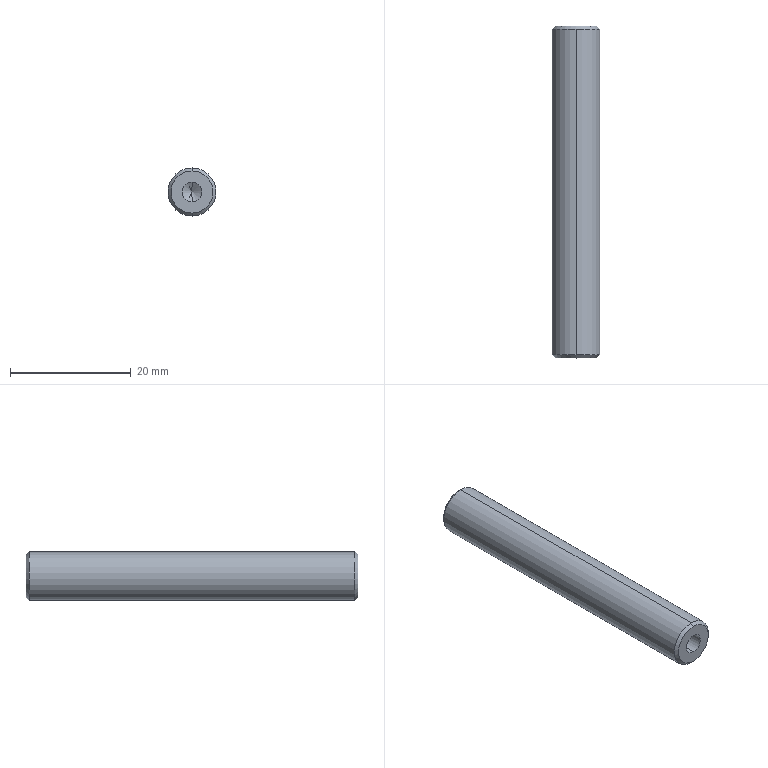Part | STEP file | PN_0012 | 1 solid | 16 faces | box 8 x 55 x 8 mm | volume 2556 mm3 | cone 8 | cylinder 6 | plane 2 | commonest cylinder face diameters 3.3 x4 8 x2
STEP:
#1=CARTESIAN_POINT('',(0.,0.,0.));
#2=DIRECTION('',(0.,0.,1.));
#3=DIRECTION('',(1.,0.,0.));
#4=AXIS2_PLACEMENT_3D('',#1,#2,#3);
#5=CARTESIAN_POINT('',(0.,27.5,3.5));
#6=VERTEX_POINT('',#5);
#7=CARTESIAN_POINT('',(0.,27.5,-3.5));
#8=VERTEX_POINT('',#7);
#9=CARTESIAN_POINT('',(0.,27.5,0.));
#10=DIRECTION('',(0.,1.,0.));
#11=DIRECTION('',(0.,0.,1.));
#12=AXIS2_PLACEMENT_3D('',#9,#10,#11);
#13=CIRCLE('',#12,3.5);
#14=CARTESIAN_POINT('',(0.,27.5,0.));
#15=DIRECTION('',(0.,-1.,0.));
#16=DIRECTION('',(0.,0.,-1.));
#17=AXIS2_PLACEMENT_3D('',#14,#15,#16);
#18=CONICAL_SURFACE('',#17,3.5,0.7854);
#19=CARTESIAN_POINT('',(3.142,0.));
#20=DIRECTION('',(-1.,0.));
#21=VECTOR('',#20,1.);
#22=LINE('',#19,#21);
#23=(GEOMETRIC_REPRESENTATION_CONTEXT(2)PARAMETRIC_REPRESENTATION_CONTEXT()REPRESENTATION_CONTEXT('',''));
#24=DEFINITIONAL_REPRESENTATION('',(#22),#23);
#25=PCURVE('',#18,#24);
#26=CARTESIAN_POINT('',(0.,27.5,0.));
#27=DIRECTION('',(0.,1.,0.));
#28=DIRECTION('',(0.,0.,1.));
#29=AXIS2_PLACEMENT_3D('',#26,#27,#28);
#30=PLANE('',#29);
#31=CARTESIAN_POINT('',(0.,0.));
#32=DIRECTION('',(1.,0.));
#33=AXIS2_PLACEMENT_2D('',#31,#32);
#34=CIRCLE('',#33,3.5);
#35=(GEOMETRIC_REPRESENTATION_CONTEXT(2)PARAMETRIC_REPRESENTATION_CONTEXT()REPRESENTATION_CONTEXT('',''));
#36=DEFINITIONAL_REPRESENTATION('',(#34),#35);
#37=PCURVE('',#30,#36);
#38=SURFACE_CURVE('',#13,(#25,#37),.PCURVE_S1.);
#39=EDGE_CURVE('',#6,#8,#38,.T.);
#40=ORIENTED_EDGE('',*,*,#39,.F.);
#41=CARTESIAN_POINT('',(0.,27.,4.));
#42=VERTEX_POINT('',#41);
#43=CARTESIAN_POINT('',(0.,27.5,3.5));
#44=DIRECTION('',(0.,-0.7071,0.7071));
#45=VECTOR('',#44,1.);
#46=LINE('',#43,#45);
#47=CARTESIAN_POINT('',(3.142,0.));
#48=DIRECTION('',(0.,1.));
#49=VECTOR('',#48,1.);
#50=LINE('',#47,#49);
#51=(GEOMETRIC_REPRESENTATION_CONTEXT(2)PARAMETRIC_REPRESENTATION_CONTEXT()REPRESENTATION_CONTEXT('',''));
#52=DEFINITIONAL_REPRESENTATION('',(#50),#51);
#53=PCURVE('',#18,#52);
#54=CARTESIAN_POINT('',(0.,27.5,0.));
#55=DIRECTION('',(0.,-1.,0.));
#56=DIRECTION('',(0.,0.,-1.));
#57=AXIS2_PLACEMENT_3D('',#54,#55,#56);
#58=CONICAL_SURFACE('',#57,3.5,0.7854);
#59=CARTESIAN_POINT('',(3.142,0.));
#60=DIRECTION('',(0.,1.));
#61=VECTOR('',#60,1.);
#62=LINE('',#59,#61);
#63=(GEOMETRIC_REPRESENTATION_CONTEXT(2)PARAMETRIC_REPRESENTATION_CONTEXT()REPRESENTATION_CONTEXT('',''));
#64=DEFINITIONAL_REPRESENTATION('',(#62),#63);
#65=PCURVE('',#58,#64);
#66=SURFACE_CURVE('',#46,(#53,#65),.PCURVE_S1.);
#67=EDGE_CURVE('',#6,#42,#66,.T.);
#68=ORIENTED_EDGE('',*,*,#67,.T.);
#69=CARTESIAN_POINT('',(0.,27.,-4.));
#70=VERTEX_POINT('',#69);
#71=CARTESIAN_POINT('',(0.,27.,0.));
#72=DIRECTION('',(0.,-1.,0.));
#73=DIRECTION('',(0.,0.,1.));
#74=AXIS2_PLACEMENT_3D('',#71,#72,#73);
#75=CIRCLE('',#74,4.);
#76=CARTESIAN_POINT('',(-3.142,0.5));
#77=DIRECTION('',(1.,0.));
#78=VECTOR('',#77,1.);
#79=LINE('',#76,#78);
#80=(GEOMETRIC_REPRESENTATION_CONTEXT(2)PARAMETRIC_REPRESENTATION_CONTEXT()REPRESENTATION_CONTEXT('',''));
#81=DEFINITIONAL_REPRESENTATION('',(#79),#80);
#82=PCURVE('',#18,#81);
#83=CARTESIAN_POINT('',(0.,27.5,0.));
#84=DIRECTION('',(0.,-1.,0.));
#85=DIRECTION('',(0.,0.,-1.));
#86=AXIS2_PLACEMENT_3D('',#83,#84,#85);
#87=CYLINDRICAL_SURFACE('',#86,4.);
#88=CARTESIAN_POINT('',(-3.142,0.5));
#89=DIRECTION('',(1.,0.));
#90=VECTOR('',#89,1.);
#91=LINE('',#88,#90);
#92=(GEOMETRIC_REPRESENTATION_CONTEXT(2)PARAMETRIC_REPRESENTATION_CONTEXT()REPRESENTATION_CONTEXT('',''));
#93=DEFINITIONAL_REPRESENTATION('',(#91),#92);
#94=PCURVE('',#87,#93);
#95=SURFACE_CURVE('',#75,(#82,#94),.PCURVE_S1.);
#96=EDGE_CURVE('',#70,#42,#95,.T.);
#97=ORIENTED_EDGE('',*,*,#96,.F.);
#98=CARTESIAN_POINT('',(0.,27.5,-3.5));
#99=DIRECTION('',(0.,-0.7071,-0.7071));
#100=VECTOR('',#99,1.);
#101=LINE('',#98,#100);
#102=CARTESIAN_POINT('',(0.,0.));
#103=DIRECTION('',(0.,1.));
#104=VECTOR('',#103,1.);
#105=LINE('',#102,#104);
#106=(GEOMETRIC_REPRESENTATION_CONTEXT(2)PARAMETRIC_REPRESENTATION_CONTEXT()REPRESENTATION_CONTEXT('',''));
#107=DEFINITIONAL_REPRESENTATION('',(#105),#106);
#108=PCURVE('',#18,#107);
#109=CARTESIAN_POINT('',(6.283,0.));
#110=DIRECTION('',(0.,1.));
#111=VECTOR('',#110,1.);
#112=LINE('',#109,#111);
#113=(GEOMETRIC_REPRESENTATION_CONTEXT(2)PARAMETRIC_REPRESENTATION_CONTEXT()REPRESENTATION_CONTEXT('',''));
#114=DEFINITIONAL_REPRESENTATION('',(#112),#113);
#115=PCURVE('',#58,#114);
#116=SURFACE_CURVE('',#101,(#108,#115),.PCURVE_S1.);
#117=EDGE_CURVE('',#8,#70,#116,.T.);
#118=ORIENTED_EDGE('',*,*,#117,.F.);
#119=EDGE_LOOP('',(#40,#68,#97,#118));
#120=FACE_BOUND('',#119,.T.);
#121=ADVANCED_FACE('',(#120),#18,.T.);
#122=CARTESIAN_POINT('',(0.,-27.5,-3.5));
#123=VERTEX_POINT('',#122);
#124=CARTESIAN_POINT('',(0.,-27.5,3.5));
#125=VERTEX_POINT('',#124);
#126=CARTESIAN_POINT('',(0.,-27.5,0.));
#127=DIRECTION('',(0.,-1.,0.));
#128=DIRECTION('',(0.,0.,1.));
#129=AXIS2_PLACEMENT_3D('',#126,#127,#128);
#130=CIRCLE('',#129,3.5);
#131=CARTESIAN_POINT('',(0.,-27.,0.));
#132=DIRECTION('',(0.,1.,0.));
#133=DIRECTION('',(0.,0.,1.));
#134=AXIS2_PLACEMENT_3D('',#131,#132,#133);
#135=CONICAL_SURFACE('',#134,4.,0.7854);
#136=CARTESIAN_POINT('',(6.283,-0.5));
#137=DIRECTION('',(-1.,0.));
#138=VECTOR('',#137,1.);
#139=LINE('',#136,#138);
#140=(GEOMETRIC_REPRESENTATION_CONTEXT(2)PARAMETRIC_REPRESENTATION_CONTEXT()REPRESENTATION_CONTEXT('',''));
#141=DEFINITIONAL_REPRESENTATION('',(#139),#140);
#142=PCURVE('',#135,#141);
#143=CARTESIAN_POINT('',(0.,-27.5,0.));
#144=DIRECTION('',(0.,1.,0.));
#145=DIRECTION('',(0.,0.,1.));
#146=AXIS2_PLACEMENT_3D('',#143,#144,#145);
#147=PLANE('',#146);
#148=CARTESIAN_POINT('',(3.5,0.));
#149=CARTESIAN_POINT('',(3.5,-6.062));
#150=CARTESIAN_POINT('',(-1.75,-3.031));
#151=CARTESIAN_POINT('',(-7.,0.));
#152=CARTESIAN_POINT('',(-1.75,3.031));
#153=CARTESIAN_POINT('',(3.5,6.062));
#154=CARTESIAN_POINT('',(3.5,0.));
#155=(BOUNDED_CURVE()B_SPLINE_CURVE(2,(#148,#149,#150,#151,#152,#153,#154),.UNSPECIFIED.,.T.,.F.)B_SPLINE_CURVE_WITH_KNOTS((1,2,2,2,2,1),(-2.094,0.,2.094,4.189,6.283,8.378),.UNSPECIFIED.)CURVE()GEOMETRIC_REPRESENTATION_ITEM()RATIONAL_B_SPLINE_CURVE((1.,0.5,1.,0.5,1.,0.5,1.))REPRESENTATION_ITEM(''));
#156=(GEOMETRIC_REPRESENTATION_CONTEXT(2)PARAMETRIC_REPRESENTATION_CONTEXT()REPRESENTATION_CONTEXT('',''));
#157=DEFINITIONAL_REPRESENTATION('',(#155),#156);
#158=PCURVE('',#147,#157);
#159=SURFACE_CURVE('',#130,(#142,#158),.PCURVE_S1.);
#160=EDGE_CURVE('',#123,#125,#159,.T.);
#161=ORIENTED_EDGE('',*,*,#160,.F.);
#162=CARTESIAN_POINT('',(0.,-27.,-4.));
#163=VERTEX_POINT('',#162);
#164=CARTESIAN_POINT('',(0.,-27.,-4.));
#165=DIRECTION('',(0.,0.7071,-0.7071));
#166=VECTOR('',#165,1.);
#167=LINE('',#164,#166);
#168=CARTESIAN_POINT('',(3.142,0.));
#169=DIRECTION('',(0.,1.));
#170=VECTOR('',#169,1.);
#171=LINE('',#168,#170);
#172=(GEOMETRIC_REPRESENTATION_CONTEXT(2)PARAMETRIC_REPRESENTATION_CONTEXT()REPRESENTATION_CONTEXT('',''));
#173=DEFINITIONAL_REPRESENTATION('',(#171),#172);
#174=PCURVE('',#135,#173);
#175=CARTESIAN_POINT('',(0.,-27.,0.));
#176=DIRECTION('',(0.,1.,0.));
#177=DIRECTION('',(0.,0.,1.));
#178=AXIS2_PLACEMENT_3D('',#175,#176,#177);
#179=CONICAL_SURFACE('',#178,4.,0.7854);
#180=CARTESIAN_POINT('',(3.142,0.));
#181=DIRECTION('',(0.,1.));
#182=VECTOR('',#181,1.);
#183=LINE('',#180,#182);
#184=(GEOMETRIC_REPRESENTATION_CONTEXT(2)PARAMETRIC_REPRESENTATION_CONTEXT()REPRESENTATION_CONTEXT('',''));
#185=DEFINITIONAL_REPRESENTATION('',(#183),#184);
#186=PCURVE('',#179,#185);
#187=SURFACE_CURVE('',#167,(#174,#186),.PCURVE_S1.);
#188=EDGE_CURVE('',#123,#163,#187,.T.);
#189=ORIENTED_EDGE('',*,*,#188,.T.);
#190=CARTESIAN_POINT('',(0.,-27.,4.));
#191=VERTEX_POINT('',#190);
#192=CARTESIAN_POINT('',(0.,-27.,0.));
#193=DIRECTION('',(0.,1.,0.));
#194=DIRECTION('',(0.,0.,1.));
#195=AXIS2_PLACEMENT_3D('',#192,#193,#194);
#196=CIRCLE('',#195,4.);
#197=CARTESIAN_POINT('',(0.,0.));
#198=DIRECTION('',(1.,0.));
#199=VECTOR('',#198,1.);
#200=LINE('',#197,#199);
#201=(GEOMETRIC_REPRESENTATION_CONTEXT(2)PARAMETRIC_REPRESENTATION_CONTEXT()REPRESENTATION_CONTEXT('',''));
#202=DEFINITIONAL_REPRESENTATION('',(#200),#201);
#203=PCURVE('',#135,#202);
#204=CARTESIAN_POINT('',(3.142,54.5));
#205=DIRECTION('',(-1.,0.));
#206=VECTOR('',#205,1.);
#207=LINE('',#204,#206);
#208=(GEOMETRIC_REPRESENTATION_CONTEXT(2)PARAMETRIC_REPRESENTATION_CONTEXT()REPRESENTATION_CONTEXT('',''));
#209=DEFINITIONAL_REPRESENTATION('',(#207),#208);
#210=PCURVE('',#87,#209);
#211=SURFACE_CURVE('',#196,(#203,#210),.PCURVE_S1.);
#212=EDGE_CURVE('',#191,#163,#211,.T.);
#213=ORIENTED_EDGE('',*,*,#212,.F.);
#214=CARTESIAN_POINT('',(0.,-27.,4.));
#215=DIRECTION('',(0.,0.7071,0.7071));
#216=VECTOR('',#215,1.);
#217=LINE('',#214,#216);
#218=CARTESIAN_POINT('',(0.,0.));
#219=DIRECTION('',(0.,1.));
#220=VECTOR('',#219,1.);
#221=LINE('',#218,#220);
#222=(GEOMETRIC_REPRESENTATION_CONTEXT(2)PARAMETRIC_REPRESENTATION_CONTEXT()REPRESENTATION_CONTEXT('',''));
#223=DEFINITIONAL_REPRESENTATION('',(#221),#222);
#224=PCURVE('',#135,#223);
#225=CARTESIAN_POINT('',(6.283,0.));
#226=DIRECTION('',(0.,1.));
#227=VECTOR('',#226,1.);
#228=LINE('',#225,#227);
#229=(GEOMETRIC_REPRESENTATION_CONTEXT(2)PARAMETRIC_REPRESENTATION_CONTEXT()REPRESENTATION_CONTEXT('',''));
#230=DEFINITIONAL_REPRESENTATION('',(#228),#229);
#231=PCURVE('',#179,#230);
#232=SURFACE_CURVE('',#217,(#224,#231),.PCURVE_S1.);
#233=EDGE_CURVE('',#125,#191,#232,.T.);
#234=ORIENTED_EDGE('',*,*,#233,.F.);
#235=EDGE_LOOP('',(#161,#189,#213,#234));
#236=FACE_BOUND('',#235,.T.);
#237=ADVANCED_FACE('',(#236),#135,.T.);
#238=CARTESIAN_POINT('',(0.,-16.,-1.65));
#239=VERTEX_POINT('',#238);
#240=CARTESIAN_POINT('',(0.,-27.5,-1.65));
#241=VERTEX_POINT('',#240);
#242=CARTESIAN_POINT('',(0.,-27.5,-1.65));
#243=DIRECTION('',(0.,-1.,0.));
#244=VECTOR('',#243,1.);
#245=LINE('',#242,#244);
#246=CARTESIAN_POINT('',(0.,-27.5,0.));
#247=DIRECTION('',(0.,-1.,0.));
#248=DIRECTION('',(0.,0.,-1.));
#249=AXIS2_PLACEMENT_3D('',#246,#247,#248);
#250=CYLINDRICAL_SURFACE('',#249,1.65);
#251=CARTESIAN_POINT('',(6.283,0.));
#252=DIRECTION('',(0.,1.));
#253=VECTOR('',#252,1.);
#254=LINE('',#251,#253);
#255=(GEOMETRIC_REPRESENTATION_CONTEXT(2)PARAMETRIC_REPRESENTATION_CONTEXT()REPRESENTATION_CONTEXT('',''));
#256=DEFINITIONAL_REPRESENTATION('',(#254),#255);
#257=PCURVE('',#250,#256);
#258=CARTESIAN_POINT('',(0.,-27.5,0.));
#259=DIRECTION('',(0.,-1.,0.));
#260=DIRECTION('',(0.,0.,-1.));
#261=AXIS2_PLACEMENT_3D('',#258,#259,#260);
#262=CYLINDRICAL_SURFACE('',#261,1.65);
#263=CARTESIAN_POINT('',(0.,0.));
#264=DIRECTION('',(0.,1.));
#265=VECTOR('',#264,1.);
#266=LINE('',#263,#265);
#267=(GEOMETRIC_REPRESENTATION_CONTEXT(2)PARAMETRIC_REPRESENTATION_CONTEXT()REPRESENTATION_CONTEXT('',''));
#268=DEFINITIONAL_REPRESENTATION('',(#266),#267);
#269=PCURVE('',#262,#268);
#270=SURFACE_CURVE('',#245,(#257,#269),.PCURVE_S1.);
#271=EDGE_CURVE('',#239,#241,#270,.T.);
#272=ORIENTED_EDGE('',*,*,#271,.T.);
#273=CARTESIAN_POINT('',(0.,-27.5,1.65));
#274=VERTEX_POINT('',#273);
#275=CARTESIAN_POINT('',(0.,-27.5,0.));
#276=DIRECTION('',(0.,-1.,0.));
#277=DIRECTION('',(0.,0.,-1.));
#278=AXIS2_PLACEMENT_3D('',#275,#276,#277);
#279=CIRCLE('',#278,1.65);
#280=CARTESIAN_POINT('',(0.,0.));
#281=DIRECTION('',(1.,0.));
#282=VECTOR('',#281,1.);
#283=LINE('',#280,#282);
#284=(GEOMETRIC_REPRESENTATION_CONTEXT(2)PARAMETRIC_REPRESENTATION_CONTEXT()REPRESENTATION_CONTEXT('',''));
#285=DEFINITIONAL_REPRESENTATION('',(#283),#284);
#286=PCURVE('',#250,#285);
#287=CARTESIAN_POINT('',(-1.65,0.));
#288=CARTESIAN_POINT('',(-1.65,2.858));
#289=CARTESIAN_POINT('',(0.825,1.429));
#290=CARTESIAN_POINT('',(3.3,0.));
#291=CARTESIAN_POINT('',(0.825,-1.429));
#292=CARTESIAN_POINT('',(-1.65,-2.858));
#293=CARTESIAN_POINT('',(-1.65,0.));
#294=(BOUNDED_CURVE()B_SPLINE_CURVE(2,(#287,#288,#289,#290,#291,#292,#293),.UNSPECIFIED.,.T.,.F.)B_SPLINE_CURVE_WITH_KNOTS((1,2,2,2,2,1),(-2.094,0.,2.094,4.189,6.283,8.378),.UNSPECIFIED.)CURVE()GEOMETRIC_REPRESENTATION_ITEM()RATIONAL_B_SPLINE_CURVE((1.,0.5,1.,0.5,1.,0.5,1.))REPRESENTATION_ITEM(''));
#295=(GEOMETRIC_REPRESENTATION_CONTEXT(2)PARAMETRIC_REPRESENTATION_CONTEXT()REPRESENTATION_CONTEXT('',''));
#296=DEFINITIONAL_REPRESENTATION('',(#294),#295);
#297=PCURVE('',#147,#296);
#298=SURFACE_CURVE('',#279,(#286,#297),.PCURVE_S1.);
#299=EDGE_CURVE('',#274,#241,#298,.T.);
#300=ORIENTED_EDGE('',*,*,#299,.F.);
#301=CARTESIAN_POINT('',(0.,-16.,1.65));
#302=VERTEX_POINT('',#301);
#303=CARTESIAN_POINT('',(0.,-27.5,1.65));
#304=DIRECTION('',(0.,-1.,0.));
#305=VECTOR('',#304,1.);
#306=LINE('',#303,#305);
#307=CARTESIAN_POINT('',(3.142,0.));
#308=DIRECTION('',(0.,1.));
#309=VECTOR('',#308,1.);
#310=LINE('',#307,#309);
#311=(GEOMETRIC_REPRESENTATION_CONTEXT(2)PARAMETRIC_REPRESENTATION_CONTEXT()REPRESENTATION_CONTEXT('',''));
#312=DEFINITIONAL_REPRESENTATION('',(#310),#311);
#313=PCURVE('',#250,#312);
#314=CARTESIAN_POINT('',(3.142,0.));
#315=DIRECTION('',(0.,1.));
#316=VECTOR('',#315,1.);
#317=LINE('',#314,#316);
#318=(GEOMETRIC_REPRESENTATION_CONTEXT(2)PARAMETRIC_REPRESENTATION_CONTEXT()REPRESENTATION_CONTEXT('',''));
#319=DEFINITIONAL_REPRESENTATION('',(#317),#318);
#320=PCURVE('',#262,#319);
#321=SURFACE_CURVE('',#306,(#313,#320),.PCURVE_S1.);
#322=EDGE_CURVE('',#302,#274,#321,.T.);
#323=ORIENTED_EDGE('',*,*,#322,.F.);
#324=CARTESIAN_POINT('',(0.,-16.,0.));
#325=DIRECTION('',(0.,-1.,0.));
#326=DIRECTION('',(0.,0.,-1.));
#327=AXIS2_PLACEMENT_3D('',#324,#325,#326);
#328=CIRCLE('',#327,1.65);
#329=CARTESIAN_POINT('',(0.,-11.5));
#330=DIRECTION('',(1.,0.));
#331=VECTOR('',#330,1.);
#332=LINE('',#329,#331);
#333=(GEOMETRIC_REPRESENTATION_CONTEXT(2)PARAMETRIC_REPRESENTATION_CONTEXT()REPRESENTATION_CONTEXT('',''));
#334=DEFINITIONAL_REPRESENTATION('',(#332),#333);
#335=PCURVE('',#250,#334);
#336=CARTESIAN_POINT('',(0.,-16.,0.));
#337=DIRECTION('',(0.,-1.,0.));
#338=DIRECTION('',(0.,0.,-1.));
#339=AXIS2_PLACEMENT_3D('',#336,#337,#338);
#340=CONICAL_SURFACE('',#339,1.65,1.03);
#341=CARTESIAN_POINT('',(0.,0.));
#342=DIRECTION('',(1.,0.));
#343=VECTOR('',#342,1.);
#344=LINE('',#341,#343);
#345=(GEOMETRIC_REPRESENTATION_CONTEXT(2)PARAMETRIC_REPRESENTATION_CONTEXT()REPRESENTATION_CONTEXT('',''));
#346=DEFINITIONAL_REPRESENTATION('',(#344),#345);
#347=PCURVE('',#340,#346);
#348=SURFACE_CURVE('',#328,(#335,#347),.PCURVE_S1.);
#349=EDGE_CURVE('',#302,#239,#348,.T.);
#350=ORIENTED_EDGE('',*,*,#349,.T.);
#351=EDGE_LOOP('',(#272,#300,#323,#350));
#352=FACE_BOUND('',#351,.F.);
#353=ADVANCED_FACE('',(#352),#250,.F.);
#354=ORIENTED_EDGE('',*,*,#349,.F.);
#355=CARTESIAN_POINT('',(0.,-15.009,0.));
#356=VERTEX_POINT('',#355);
#357=CARTESIAN_POINT('',(0.,-16.,1.65));
#358=DIRECTION('',(0.,-0.515,0.8572));
#359=VECTOR('',#358,1.);
#360=LINE('',#357,#359);
#361=CARTESIAN_POINT('',(3.142,0.));
#362=DIRECTION('',(0.,1.));
#363=VECTOR('',#362,1.);
#364=LINE('',#361,#363);
#365=(GEOMETRIC_REPRESENTATION_CONTEXT(2)PARAMETRIC_REPRESENTATION_CONTEXT()REPRESENTATION_CONTEXT('',''));
#366=DEFINITIONAL_REPRESENTATION('',(#364),#365);
#367=PCURVE('',#340,#366);
#368=CARTESIAN_POINT('',(0.,-16.,0.));
#369=DIRECTION('',(0.,-1.,0.));
#370=DIRECTION('',(0.,0.,-1.));
#371=AXIS2_PLACEMENT_3D('',#368,#369,#370);
#372=CONICAL_SURFACE('',#371,1.65,1.03);
#373=CARTESIAN_POINT('',(3.142,0.));
#374=DIRECTION('',(0.,1.));
#375=VECTOR('',#374,1.);
#376=LINE('',#373,#375);
#377=(GEOMETRIC_REPRESENTATION_CONTEXT(2)PARAMETRIC_REPRESENTATION_CONTEXT()REPRESENTATION_CONTEXT('',''));
#378=DEFINITIONAL_REPRESENTATION('',(#376),#377);
#379=PCURVE('',#372,#378);
#380=SURFACE_CURVE('',#360,(#367,#379),.PCURVE_S1.);
#381=EDGE_CURVE('',#356,#302,#380,.T.);
#382=ORIENTED_EDGE('',*,*,#381,.F.);
#383=CARTESIAN_POINT('',(0.,-16.,-1.65));
#384=DIRECTION('',(0.,-0.515,-0.8572));
#385=VECTOR('',#384,1.);
#386=LINE('',#383,#385);
#387=CARTESIAN_POINT('',(6.283,0.));
#388=DIRECTION('',(0.,1.));
#389=VECTOR('',#388,1.);
#390=LINE('',#387,#389);
#391=(GEOMETRIC_REPRESENTATION_CONTEXT(2)PARAMETRIC_REPRESENTATION_CONTEXT()REPRESENTATION_CONTEXT('',''));
#392=DEFINITIONAL_REPRESENTATION('',(#390),#391);
#393=PCURVE('',#340,#392);
#394=CARTESIAN_POINT('',(0.,0.));
#395=DIRECTION('',(0.,1.));
#396=VECTOR('',#395,1.);
#397=LINE('',#394,#396);
#398=(GEOMETRIC_REPRESENTATION_CONTEXT(2)PARAMETRIC_REPRESENTATION_CONTEXT()REPRESENTATION_CONTEXT('',''));
#399=DEFINITIONAL_REPRESENTATION('',(#397),#398);
#400=PCURVE('',#372,#399);
#401=SURFACE_CURVE('',#386,(#393,#400),.PCURVE_S1.);
#402=EDGE_CURVE('',#356,#239,#401,.T.);
#403=ORIENTED_EDGE('',*,*,#402,.T.);
#404=EDGE_LOOP('',(#354,#382,#403));
#405=FACE_BOUND('',#404,.F.);
#406=ADVANCED_FACE('',(#405),#340,.F.);
#407=CARTESIAN_POINT('',(0.,16.,1.65));
#408=VERTEX_POINT('',#407);
#409=CARTESIAN_POINT('',(0.,27.5,1.65));
#410=VERTEX_POINT('',#409);
#411=CARTESIAN_POINT('',(0.,27.5,1.65));
#412=DIRECTION('',(0.,1.,0.));
#413=VECTOR('',#412,1.);
#414=LINE('',#411,#413);
#415=CARTESIAN_POINT('',(0.,27.5,0.));
#416=DIRECTION('',(0.,1.,0.));
#417=DIRECTION('',(0.,0.,1.));
#418=AXIS2_PLACEMENT_3D('',#415,#416,#417);
#419=CYLINDRICAL_SURFACE('',#418,1.65);
#420=CARTESIAN_POINT('',(6.283,0.));
#421=DIRECTION('',(0.,1.));
#422=VECTOR('',#421,1.);
#423=LINE('',#420,#422);
#424=(GEOMETRIC_REPRESENTATION_CONTEXT(2)PARAMETRIC_REPRESENTATION_CONTEXT()REPRESENTATION_CONTEXT('',''));
#425=DEFINITIONAL_REPRESENTATION('',(#423),#424);
#426=PCURVE('',#419,#425);
#427=CARTESIAN_POINT('',(0.,27.5,0.));
#428=DIRECTION('',(0.,1.,0.));
#429=DIRECTION('',(0.,0.,1.));
#430=AXIS2_PLACEMENT_3D('',#427,#428,#429);
#431=CYLINDRICAL_SURFACE('',#430,1.65);
#432=CARTESIAN_POINT('',(0.,0.));
#433=DIRECTION('',(0.,1.));
#434=VECTOR('',#433,1.);
#435=LINE('',#432,#434);
#436=(GEOMETRIC_REPRESENTATION_CONTEXT(2)PARAMETRIC_REPRESENTATION_CONTEXT()REPRESENTATION_CONTEXT('',''));
#437=DEFINITIONAL_REPRESENTATION('',(#435),#436);
#438=PCURVE('',#431,#437);
#439=SURFACE_CURVE('',#414,(#426,#438),.PCURVE_S1.);
#440=EDGE_CURVE('',#408,#410,#439,.T.);
#441=ORIENTED_EDGE('',*,*,#440,.T.);
#442=CARTESIAN_POINT('',(0.,27.5,-1.65));
#443=VERTEX_POINT('',#442);
#444=CARTESIAN_POINT('',(0.,27.5,0.));
#445=DIRECTION('',(0.,1.,0.));
#446=DIRECTION('',(0.,0.,1.));
#447=AXIS2_PLACEMENT_3D('',#444,#445,#446);
#448=CIRCLE('',#447,1.65);
#449=CARTESIAN_POINT('',(0.,0.));
#450=DIRECTION('',(1.,0.));
#451=VECTOR('',#450,1.);
#452=LINE('',#449,#451);
#453=(GEOMETRIC_REPRESENTATION_CONTEXT(2)PARAMETRIC_REPRESENTATION_CONTEXT()REPRESENTATION_CONTEXT('',''));
#454=DEFINITIONAL_REPRESENTATION('',(#452),#453);
#455=PCURVE('',#419,#454);
#456=CARTESIAN_POINT('',(0.,0.));
#457=DIRECTION('',(1.,0.));
#458=AXIS2_PLACEMENT_2D('',#456,#457);
#459=CIRCLE('',#458,1.65);
#460=(GEOMETRIC_REPRESENTATION_CONTEXT(2)PARAMETRIC_REPRESENTATION_CONTEXT()REPRESENTATION_CONTEXT('',''));
#461=DEFINITIONAL_REPRESENTATION('',(#459),#460);
#462=PCURVE('',#30,#461);
#463=SURFACE_CURVE('',#448,(#455,#462),.PCURVE_S1.);
#464=EDGE_CURVE('',#443,#410,#463,.T.);
#465=ORIENTED_EDGE('',*,*,#464,.F.);
#466=CARTESIAN_POINT('',(0.,16.,-1.65));
#467=VERTEX_POINT('',#466);
#468=CARTESIAN_POINT('',(0.,27.5,-1.65));
#469=DIRECTION('',(0.,1.,0.));
#470=VECTOR('',#469,1.);
#471=LINE('',#468,#470);
#472=CARTESIAN_POINT('',(3.142,0.));
#473=DIRECTION('',(0.,1.));
#474=VECTOR('',#473,1.);
#475=LINE('',#472,#474);
#476=(GEOMETRIC_REPRESENTATION_CONTEXT(2)PARAMETRIC_REPRESENTATION_CONTEXT()REPRESENTATION_CONTEXT('',''));
#477=DEFINITIONAL_REPRESENTATION('',(#475),#476);
#478=PCURVE('',#419,#477);
#479=CARTESIAN_POINT('',(3.142,0.));
#480=DIRECTION('',(0.,1.));
#481=VECTOR('',#480,1.);
#482=LINE('',#479,#481);
#483=(GEOMETRIC_REPRESENTATION_CONTEXT(2)PARAMETRIC_REPRESENTATION_CONTEXT()REPRESENTATION_CONTEXT('',''));
#484=DEFINITIONAL_REPRESENTATION('',(#482),#483);
#485=PCURVE('',#431,#484);
#486=SURFACE_CURVE('',#471,(#478,#485),.PCURVE_S1.);
#487=EDGE_CURVE('',#467,#443,#486,.T.);
#488=ORIENTED_EDGE('',*,*,#487,.F.);
#489=CARTESIAN_POINT('',(0.,16.,0.));
#490=DIRECTION('',(0.,1.,0.));
#491=DIRECTION('',(0.,0.,1.));
#492=AXIS2_PLACEMENT_3D('',#489,#490,#491);
#493=CIRCLE('',#492,1.65);
#494=CARTESIAN_POINT('',(0.,-11.5));
#495=DIRECTION('',(1.,0.));
#496=VECTOR('',#495,1.);
#497=LINE('',#494,#496);
#498=(GEOMETRIC_REPRESENTATION_CONTEXT(2)PARAMETRIC_REPRESENTATION_CONTEXT()REPRESENTATION_CONTEXT('',''));
#499=DEFINITIONAL_REPRESENTATION('',(#497),#498);
#500=PCURVE('',#419,#499);
#501=CARTESIAN_POINT('',(0.,16.,0.));
#502=DIRECTION('',(0.,1.,0.));
#503=DIRECTION('',(0.,0.,1.));
#504=AXIS2_PLACEMENT_3D('',#501,#502,#503);
#505=CONICAL_SURFACE('',#504,1.65,1.03);
#506=CARTESIAN_POINT('',(0.,0.));
#507=DIRECTION('',(1.,0.));
#508=VECTOR('',#507,1.);
#509=LINE('',#506,#508);
#510=(GEOMETRIC_REPRESENTATION_CONTEXT(2)PARAMETRIC_REPRESENTATION_CONTEXT()REPRESENTATION_CONTEXT('',''));
#511=DEFINITIONAL_REPRESENTATION('',(#509),#510);
#512=PCURVE('',#505,#511);
#513=SURFACE_CURVE('',#493,(#500,#512),.PCURVE_S1.);
#514=EDGE_CURVE('',#467,#408,#513,.T.);
#515=ORIENTED_EDGE('',*,*,#514,.T.);
#516=EDGE_LOOP('',(#441,#465,#488,#515));
#517=FACE_BOUND('',#516,.F.);
#518=ADVANCED_FACE('',(#517),#419,.F.);
#519=ORIENTED_EDGE('',*,*,#514,.F.);
#520=CARTESIAN_POINT('',(0.,15.009,0.));
#521=VERTEX_POINT('',#520);
#522=CARTESIAN_POINT('',(0.,16.,-1.65));
#523=DIRECTION('',(0.,0.515,-0.8572));
#524=VECTOR('',#523,1.);
#525=LINE('',#522,#524);
#526=CARTESIAN_POINT('',(3.142,0.));
#527=DIRECTION('',(0.,1.));
#528=VECTOR('',#527,1.);
#529=LINE('',#526,#528);
#530=(GEOMETRIC_REPRESENTATION_CONTEXT(2)PARAMETRIC_REPRESENTATION_CONTEXT()REPRESENTATION_CONTEXT('',''));
#531=DEFINITIONAL_REPRESENTATION('',(#529),#530);
#532=PCURVE('',#505,#531);
#533=CARTESIAN_POINT('',(0.,16.,0.));
#534=DIRECTION('',(0.,1.,0.));
#535=DIRECTION('',(0.,0.,1.));
#536=AXIS2_PLACEMENT_3D('',#533,#534,#535);
#537=CONICAL_SURFACE('',#536,1.65,1.03);
#538=CARTESIAN_POINT('',(3.142,0.));
#539=DIRECTION('',(0.,1.));
#540=VECTOR('',#539,1.);
#541=LINE('',#538,#540);
#542=(GEOMETRIC_REPRESENTATION_CONTEXT(2)PARAMETRIC_REPRESENTATION_CONTEXT()REPRESENTATION_CONTEXT('',''));
#543=DEFINITIONAL_REPRESENTATION('',(#541),#542);
#544=PCURVE('',#537,#543);
#545=SURFACE_CURVE('',#525,(#532,#544),.PCURVE_S1.);
#546=EDGE_CURVE('',#521,#467,#545,.T.);
#547=ORIENTED_EDGE('',*,*,#546,.F.);
#548=CARTESIAN_POINT('',(0.,16.,1.65));
#549=DIRECTION('',(0.,0.515,0.8572));
#550=VECTOR('',#549,1.);
#551=LINE('',#548,#550);
#552=CARTESIAN_POINT('',(6.283,0.));
#553=DIRECTION('',(0.,1.));
#554=VECTOR('',#553,1.);
#555=LINE('',#552,#554);
#556=(GEOMETRIC_REPRESENTATION_CONTEXT(2)PARAMETRIC_REPRESENTATION_CONTEXT()REPRESENTATION_CONTEXT('',''));
#557=DEFINITIONAL_REPRESENTATION('',(#555),#556);
#558=PCURVE('',#505,#557);
#559=CARTESIAN_POINT('',(0.,0.));
#560=DIRECTION('',(0.,1.));
#561=VECTOR('',#560,1.);
#562=LINE('',#559,#561);
#563=(GEOMETRIC_REPRESENTATION_CONTEXT(2)PARAMETRIC_REPRESENTATION_CONTEXT()REPRESENTATION_CONTEXT('',''));
#564=DEFINITIONAL_REPRESENTATION('',(#562),#563);
#565=PCURVE('',#537,#564);
#566=SURFACE_CURVE('',#551,(#558,#565),.PCURVE_S1.);
#567=EDGE_CURVE('',#521,#408,#566,.T.);
#568=ORIENTED_EDGE('',*,*,#567,.T.);
#569=EDGE_LOOP('',(#519,#547,#568));
#570=FACE_BOUND('',#569,.F.);
#571=ADVANCED_FACE('',(#570),#505,.F.);
#572=ORIENTED_EDGE('',*,*,#96,.T.);
#573=CARTESIAN_POINT('',(0.,27.5,4.));
#574=DIRECTION('',(0.,-1.,0.));
#575=VECTOR('',#574,1.);
#576=LINE('',#573,#575);
#577=CARTESIAN_POINT('',(3.142,0.));
#578=DIRECTION('',(0.,1.));
#579=VECTOR('',#578,1.);
#580=LINE('',#577,#579);
#581=(GEOMETRIC_REPRESENTATION_CONTEXT(2)PARAMETRIC_REPRESENTATION_CONTEXT()REPRESENTATION_CONTEXT('',''));
#582=DEFINITIONAL_REPRESENTATION('',(#580),#581);
#583=PCURVE('',#87,#582);
#584=CARTESIAN_POINT('',(0.,27.5,0.));
#585=DIRECTION('',(0.,-1.,0.));
#586=DIRECTION('',(0.,0.,-1.));
#587=AXIS2_PLACEMENT_3D('',#584,#585,#586);
#588=CYLINDRICAL_SURFACE('',#587,4.);
#589=CARTESIAN_POINT('',(3.142,0.));
#590=DIRECTION('',(0.,1.));
#591=VECTOR('',#590,1.);
#592=LINE('',#589,#591);
#593=(GEOMETRIC_REPRESENTATION_CONTEXT(2)PARAMETRIC_REPRESENTATION_CONTEXT()REPRESENTATION_CONTEXT('',''));
#594=DEFINITIONAL_REPRESENTATION('',(#592),#593);
#595=PCURVE('',#588,#594);
#596=SURFACE_CURVE('',#576,(#583,#595),.PCURVE_S1.);
#597=EDGE_CURVE('',#42,#191,#596,.T.);
#598=ORIENTED_EDGE('',*,*,#597,.T.);
#599=ORIENTED_EDGE('',*,*,#212,.T.);
#600=CARTESIAN_POINT('',(0.,27.5,-4.));
#601=DIRECTION('',(0.,-1.,0.));
#602=VECTOR('',#601,1.);
#603=LINE('',#600,#602);
#604=CARTESIAN_POINT('',(0.,0.));
#605=DIRECTION('',(0.,1.));
#606=VECTOR('',#605,1.);
#607=LINE('',#604,#606);
#608=(GEOMETRIC_REPRESENTATION_CONTEXT(2)PARAMETRIC_REPRESENTATION_CONTEXT()REPRESENTATION_CONTEXT('',''));
#609=DEFINITIONAL_REPRESENTATION('',(#607),#608);
#610=PCURVE('',#87,#609);
#611=CARTESIAN_POINT('',(6.283,0.));
#612=DIRECTION('',(0.,1.));
#613=VECTOR('',#612,1.);
#614=LINE('',#611,#613);
#615=(GEOMETRIC_REPRESENTATION_CONTEXT(2)PARAMETRIC_REPRESENTATION_CONTEXT()REPRESENTATION_CONTEXT('',''));
#616=DEFINITIONAL_REPRESENTATION('',(#614),#615);
#617=PCURVE('',#588,#616);
#618=SURFACE_CURVE('',#603,(#610,#617),.PCURVE_S1.);
#619=EDGE_CURVE('',#70,#163,#618,.T.);
#620=ORIENTED_EDGE('',*,*,#619,.F.);
#621=EDGE_LOOP('',(#572,#598,#599,#620));
#622=FACE_BOUND('',#621,.T.);
#623=ADVANCED_FACE('',(#622),#87,.T.);
#624=ORIENTED_EDGE('',*,*,#597,.F.);
#625=CARTESIAN_POINT('',(0.,27.,0.));
#626=DIRECTION('',(0.,-1.,0.));
#627=DIRECTION('',(0.,0.,1.));
#628=AXIS2_PLACEMENT_3D('',#625,#626,#627);
#629=CIRCLE('',#628,4.);
#630=CARTESIAN_POINT('',(3.142,0.5));
#631=DIRECTION('',(1.,0.));
#632=VECTOR('',#631,1.);
#633=LINE('',#630,#632);
#634=(GEOMETRIC_REPRESENTATION_CONTEXT(2)PARAMETRIC_REPRESENTATION_CONTEXT()REPRESENTATION_CONTEXT('',''));
#635=DEFINITIONAL_REPRESENTATION('',(#633),#634);
#636=PCURVE('',#588,#635);
#637=CARTESIAN_POINT('',(3.142,0.5));
#638=DIRECTION('',(1.,0.));
#639=VECTOR('',#638,1.);
#640=LINE('',#637,#639);
#641=(GEOMETRIC_REPRESENTATION_CONTEXT(2)PARAMETRIC_REPRESENTATION_CONTEXT()REPRESENTATION_CONTEXT('',''));
#642=DEFINITIONAL_REPRESENTATION('',(#640),#641);
#643=PCURVE('',#58,#642);
#644=SURFACE_CURVE('',#629,(#636,#643),.PCURVE_S1.);
#645=EDGE_CURVE('',#42,#70,#644,.T.);
#646=ORIENTED_EDGE('',*,*,#645,.T.);
#647=ORIENTED_EDGE('',*,*,#619,.T.);
#648=CARTESIAN_POINT('',(0.,-27.,0.));
#649=DIRECTION('',(0.,1.,0.));
#650=DIRECTION('',(0.,0.,1.));
#651=AXIS2_PLACEMENT_3D('',#648,#649,#650);
#652=CIRCLE('',#651,4.);
#653=CARTESIAN_POINT('',(9.425,54.5));
#654=DIRECTION('',(-1.,0.));
#655=VECTOR('',#654,1.);
#656=LINE('',#653,#655);
#657=(GEOMETRIC_REPRESENTATION_CONTEXT(2)PARAMETRIC_REPRESENTATION_CONTEXT()REPRESENTATION_CONTEXT('',''));
#658=DEFINITIONAL_REPRESENTATION('',(#656),#657);
#659=PCURVE('',#588,#658);
#660=CARTESIAN_POINT('',(0.,0.));
#661=DIRECTION('',(1.,0.));
#662=VECTOR('',#661,1.);
#663=LINE('',#660,#662);
#664=(GEOMETRIC_REPRESENTATION_CONTEXT(2)PARAMETRIC_REPRESENTATION_CONTEXT()REPRESENTATION_CONTEXT('',''));
#665=DEFINITIONAL_REPRESENTATION('',(#663),#664);
#666=PCURVE('',#179,#665);
#667=SURFACE_CURVE('',#652,(#659,#666),.PCURVE_S1.);
#668=EDGE_CURVE('',#163,#191,#667,.T.);
#669=ORIENTED_EDGE('',*,*,#668,.T.);
#670=EDGE_LOOP('',(#624,#646,#647,#669));
#671=FACE_BOUND('',#670,.T.);
#672=ADVANCED_FACE('',(#671),#588,.T.);
#673=CARTESIAN_POINT('',(0.,27.5,0.));
#674=DIRECTION('',(0.,1.,0.));
#675=DIRECTION('',(0.,0.,1.));
#676=AXIS2_PLACEMENT_3D('',#673,#674,#675);
#677=CIRCLE('',#676,3.5);
#678=CARTESIAN_POINT('',(0.,0.));
#679=DIRECTION('',(1.,0.));
#680=AXIS2_PLACEMENT_2D('',#678,#679);
#681=CIRCLE('',#680,3.5);
#682=(GEOMETRIC_REPRESENTATION_CONTEXT(2)PARAMETRIC_REPRESENTATION_CONTEXT()REPRESENTATION_CONTEXT('',''));
#683=DEFINITIONAL_REPRESENTATION('',(#681),#682);
#684=PCURVE('',#30,#683);
#685=CARTESIAN_POINT('',(9.425,0.));
#686=DIRECTION('',(-1.,0.));
#687=VECTOR('',#686,1.);
#688=LINE('',#685,#687);
#689=(GEOMETRIC_REPRESENTATION_CONTEXT(2)PARAMETRIC_REPRESENTATION_CONTEXT()REPRESENTATION_CONTEXT('',''));
#690=DEFINITIONAL_REPRESENTATION('',(#688),#689);
#691=PCURVE('',#58,#690);
#692=SURFACE_CURVE('',#677,(#684,#691),.PCURVE_S1.);
#693=EDGE_CURVE('',#8,#6,#692,.T.);
#694=ORIENTED_EDGE('',*,*,#693,.T.);
#695=ORIENTED_EDGE('',*,*,#39,.T.);
#696=EDGE_LOOP('',(#694,#695));
#697=FACE_BOUND('',#696,.T.);
#698=CARTESIAN_POINT('',(0.,27.5,0.));
#699=DIRECTION('',(0.,1.,0.));
#700=DIRECTION('',(0.,0.,1.));
#701=AXIS2_PLACEMENT_3D('',#698,#699,#700);
#702=CIRCLE('',#701,1.65);
#703=CARTESIAN_POINT('',(0.,0.));
#704=DIRECTION('',(1.,0.));
#705=AXIS2_PLACEMENT_2D('',#703,#704);
#706=CIRCLE('',#705,1.65);
#707=(GEOMETRIC_REPRESENTATION_CONTEXT(2)PARAMETRIC_REPRESENTATION_CONTEXT()REPRESENTATION_CONTEXT('',''));
#708=DEFINITIONAL_REPRESENTATION('',(#706),#707);
#709=PCURVE('',#30,#708);
#710=CARTESIAN_POINT('',(0.,0.));
#711=DIRECTION('',(1.,0.));
#712=VECTOR('',#711,1.);
#713=LINE('',#710,#712);
#714=(GEOMETRIC_REPRESENTATION_CONTEXT(2)PARAMETRIC_REPRESENTATION_CONTEXT()REPRESENTATION_CONTEXT('',''));
#715=DEFINITIONAL_REPRESENTATION('',(#713),#714);
#716=PCURVE('',#431,#715);
#717=SURFACE_CURVE('',#702,(#709,#716),.PCURVE_S1.);
#718=EDGE_CURVE('',#410,#443,#717,.T.);
#719=ORIENTED_EDGE('',*,*,#718,.F.);
#720=ORIENTED_EDGE('',*,*,#464,.F.);
#721=EDGE_LOOP('',(#719,#720));
#722=FACE_BOUND('',#721,.T.);
#723=ADVANCED_FACE('',(#697,#722),#30,.T.);
#724=CARTESIAN_POINT('',(0.,-27.5,0.));
#725=DIRECTION('',(0.,-1.,0.));
#726=DIRECTION('',(0.,0.,1.));
#727=AXIS2_PLACEMENT_3D('',#724,#725,#726);
#728=CIRCLE('',#727,3.5);
#729=CARTESIAN_POINT('',(3.5,0.));
#730=CARTESIAN_POINT('',(3.5,-6.062));
#731=CARTESIAN_POINT('',(-1.75,-3.031));
#732=CARTESIAN_POINT('',(-7.,0.));
#733=CARTESIAN_POINT('',(-1.75,3.031));
#734=CARTESIAN_POINT('',(3.5,6.062));
#735=CARTESIAN_POINT('',(3.5,0.));
#736=(BOUNDED_CURVE()B_SPLINE_CURVE(2,(#729,#730,#731,#732,#733,#734,#735),.UNSPECIFIED.,.T.,.F.)B_SPLINE_CURVE_WITH_KNOTS((1,2,2,2,2,1),(-2.094,0.,2.094,4.189,6.283,8.378),.UNSPECIFIED.)CURVE()GEOMETRIC_REPRESENTATION_ITEM()RATIONAL_B_SPLINE_CURVE((1.,0.5,1.,0.5,1.,0.5,1.))REPRESENTATION_ITEM(''));
#737=(GEOMETRIC_REPRESENTATION_CONTEXT(2)PARAMETRIC_REPRESENTATION_CONTEXT()REPRESENTATION_CONTEXT('',''));
#738=DEFINITIONAL_REPRESENTATION('',(#736),#737);
#739=PCURVE('',#147,#738);
#740=CARTESIAN_POINT('',(6.283,-0.5));
#741=DIRECTION('',(-1.,0.));
#742=VECTOR('',#741,1.);
#743=LINE('',#740,#742);
#744=(GEOMETRIC_REPRESENTATION_CONTEXT(2)PARAMETRIC_REPRESENTATION_CONTEXT()REPRESENTATION_CONTEXT('',''));
#745=DEFINITIONAL_REPRESENTATION('',(#743),#744);
#746=PCURVE('',#179,#745);
#747=SURFACE_CURVE('',#728,(#739,#746),.PCURVE_S1.);
#748=EDGE_CURVE('',#125,#123,#747,.T.);
#749=ORIENTED_EDGE('',*,*,#748,.T.);
#750=ORIENTED_EDGE('',*,*,#160,.T.);
#751=EDGE_LOOP('',(#749,#750));
#752=FACE_BOUND('',#751,.T.);
#753=CARTESIAN_POINT('',(0.,-27.5,0.));
#754=DIRECTION('',(0.,-1.,0.));
#755=DIRECTION('',(0.,0.,-1.));
#756=AXIS2_PLACEMENT_3D('',#753,#754,#755);
#757=CIRCLE('',#756,1.65);
#758=CARTESIAN_POINT('',(-1.65,0.));
#759=CARTESIAN_POINT('',(-1.65,2.858));
#760=CARTESIAN_POINT('',(0.825,1.429));
#761=CARTESIAN_POINT('',(3.3,0.));
#762=CARTESIAN_POINT('',(0.825,-1.429));
#763=CARTESIAN_POINT('',(-1.65,-2.858));
#764=CARTESIAN_POINT('',(-1.65,0.));
#765=(BOUNDED_CURVE()B_SPLINE_CURVE(2,(#758,#759,#760,#761,#762,#763,#764),.UNSPECIFIED.,.T.,.F.)B_SPLINE_CURVE_WITH_KNOTS((1,2,2,2,2,1),(-2.094,0.,2.094,4.189,6.283,8.378),.UNSPECIFIED.)CURVE()GEOMETRIC_REPRESENTATION_ITEM()RATIONAL_B_SPLINE_CURVE((1.,0.5,1.,0.5,1.,0.5,1.))REPRESENTATION_ITEM(''));
#766=(GEOMETRIC_REPRESENTATION_CONTEXT(2)PARAMETRIC_REPRESENTATION_CONTEXT()REPRESENTATION_CONTEXT('',''));
#767=DEFINITIONAL_REPRESENTATION('',(#765),#766);
#768=PCURVE('',#147,#767);
#769=CARTESIAN_POINT('',(0.,0.));
#770=DIRECTION('',(1.,0.));
#771=VECTOR('',#770,1.);
#772=LINE('',#769,#771);
#773=(GEOMETRIC_REPRESENTATION_CONTEXT(2)PARAMETRIC_REPRESENTATION_CONTEXT()REPRESENTATION_CONTEXT('',''));
#774=DEFINITIONAL_REPRESENTATION('',(#772),#773);
#775=PCURVE('',#262,#774);
#776=SURFACE_CURVE('',#757,(#768,#775),.PCURVE_S1.);
#777=EDGE_CURVE('',#241,#274,#776,.T.);
#778=ORIENTED_EDGE('',*,*,#777,.F.);
#779=ORIENTED_EDGE('',*,*,#299,.F.);
#780=EDGE_LOOP('',(#778,#779));
#781=FACE_BOUND('',#780,.T.);
#782=ADVANCED_FACE('',(#752,#781),#147,.F.);
#783=CARTESIAN_POINT('',(0.,16.,0.));
#784=DIRECTION('',(0.,1.,0.));
#785=DIRECTION('',(0.,0.,1.));
#786=AXIS2_PLACEMENT_3D('',#783,#784,#785);
#787=CIRCLE('',#786,1.65);
#788=CARTESIAN_POINT('',(0.,0.));
#789=DIRECTION('',(1.,0.));
#790=VECTOR('',#789,1.);
#791=LINE('',#788,#790);
#792=(GEOMETRIC_REPRESENTATION_CONTEXT(2)PARAMETRIC_REPRESENTATION_CONTEXT()REPRESENTATION_CONTEXT('',''));
#793=DEFINITIONAL_REPRESENTATION('',(#791),#792);
#794=PCURVE('',#537,#793);
#795=CARTESIAN_POINT('',(0.,-11.5));
#796=DIRECTION('',(1.,0.));
#797=VECTOR('',#796,1.);
#798=LINE('',#795,#797);
#799=(GEOMETRIC_REPRESENTATION_CONTEXT(2)PARAMETRIC_REPRESENTATION_CONTEXT()REPRESENTATION_CONTEXT('',''));
#800=DEFINITIONAL_REPRESENTATION('',(#798),#799);
#801=PCURVE('',#431,#800);
#802=SURFACE_CURVE('',#787,(#794,#801),.PCURVE_S1.);
#803=EDGE_CURVE('',#408,#467,#802,.T.);
#804=ORIENTED_EDGE('',*,*,#803,.F.);
#805=ORIENTED_EDGE('',*,*,#567,.F.);
#806=ORIENTED_EDGE('',*,*,#546,.T.);
#807=EDGE_LOOP('',(#804,#805,#806));
#808=FACE_BOUND('',#807,.F.);
#809=ADVANCED_FACE('',(#808),#537,.F.);
#810=ORIENTED_EDGE('',*,*,#718,.F.);
#811=ORIENTED_EDGE('',*,*,#440,.F.);
#812=ORIENTED_EDGE('',*,*,#803,.T.);
#813=ORIENTED_EDGE('',*,*,#487,.T.);
#814=EDGE_LOOP('',(#810,#811,#812,#813));
#815=FACE_BOUND('',#814,.F.);
#816=ADVANCED_FACE('',(#815),#431,.F.);
#817=CARTESIAN_POINT('',(0.,-16.,0.));
#818=DIRECTION('',(0.,-1.,0.));
#819=DIRECTION('',(0.,0.,-1.));
#820=AXIS2_PLACEMENT_3D('',#817,#818,#819);
#821=CIRCLE('',#820,1.65);
#822=CARTESIAN_POINT('',(0.,0.));
#823=DIRECTION('',(1.,0.));
#824=VECTOR('',#823,1.);
#825=LINE('',#822,#824);
#826=(GEOMETRIC_REPRESENTATION_CONTEXT(2)PARAMETRIC_REPRESENTATION_CONTEXT()REPRESENTATION_CONTEXT('',''));
#827=DEFINITIONAL_REPRESENTATION('',(#825),#826);
#828=PCURVE('',#372,#827);
#829=CARTESIAN_POINT('',(0.,-11.5));
#830=DIRECTION('',(1.,0.));
#831=VECTOR('',#830,1.);
#832=LINE('',#829,#831);
#833=(GEOMETRIC_REPRESENTATION_CONTEXT(2)PARAMETRIC_REPRESENTATION_CONTEXT()REPRESENTATION_CONTEXT('',''));
#834=DEFINITIONAL_REPRESENTATION('',(#832),#833);
#835=PCURVE('',#262,#834);
#836=SURFACE_CURVE('',#821,(#828,#835),.PCURVE_S1.);
#837=EDGE_CURVE('',#239,#302,#836,.T.);
#838=ORIENTED_EDGE('',*,*,#837,.F.);
#839=ORIENTED_EDGE('',*,*,#402,.F.);
#840=ORIENTED_EDGE('',*,*,#381,.T.);
#841=EDGE_LOOP('',(#838,#839,#840));
#842=FACE_BOUND('',#841,.F.);
#843=ADVANCED_FACE('',(#842),#372,.F.);
#844=ORIENTED_EDGE('',*,*,#777,.F.);
#845=ORIENTED_EDGE('',*,*,#271,.F.);
#846=ORIENTED_EDGE('',*,*,#837,.T.);
#847=ORIENTED_EDGE('',*,*,#322,.T.);
#848=EDGE_LOOP('',(#844,#845,#846,#847));
#849=FACE_BOUND('',#848,.F.);
#850=ADVANCED_FACE('',(#849),#262,.F.);
#851=ORIENTED_EDGE('',*,*,#188,.F.);
#852=ORIENTED_EDGE('',*,*,#748,.F.);
#853=ORIENTED_EDGE('',*,*,#233,.T.);
#854=ORIENTED_EDGE('',*,*,#668,.F.);
#855=EDGE_LOOP('',(#851,#852,#853,#854));
#856=FACE_BOUND('',#855,.T.);
#857=ADVANCED_FACE('',(#856),#179,.T.);
#858=ORIENTED_EDGE('',*,*,#67,.F.);
#859=ORIENTED_EDGE('',*,*,#693,.F.);
#860=ORIENTED_EDGE('',*,*,#117,.T.);
#861=ORIENTED_EDGE('',*,*,#645,.F.);
#862=EDGE_LOOP('',(#858,#859,#860,#861));
#863=FACE_BOUND('',#862,.T.);
#864=ADVANCED_FACE('',(#863),#58,.T.);
#865=CLOSED_SHELL('',(#121,#237,#353,#406,#518,#571,#623,#672,#723,#782,#809,#816,#843,#850,#857,#864));
#866=MANIFOLD_SOLID_BREP('',#865);
#867=(LENGTH_UNIT()NAMED_UNIT(*)SI_UNIT(.MILLI.,.METRE.));
#868=UNCERTAINTY_MEASURE_WITH_UNIT(LENGTH_MEASURE(0.0000001),#867,'','');
#869=(NAMED_UNIT(*)PLANE_ANGLE_UNIT()SI_UNIT($,.RADIAN.));
#870=(NAMED_UNIT(*)SI_UNIT($,.STERADIAN.)SOLID_ANGLE_UNIT());
#871=(GEOMETRIC_REPRESENTATION_CONTEXT(3)GLOBAL_UNCERTAINTY_ASSIGNED_CONTEXT((#868))GLOBAL_UNIT_ASSIGNED_CONTEXT((#867,#869,#870))REPRESENTATION_CONTEXT('',''));
#872=ADVANCED_BREP_SHAPE_REPRESENTATION('',(#4,#866),#871);